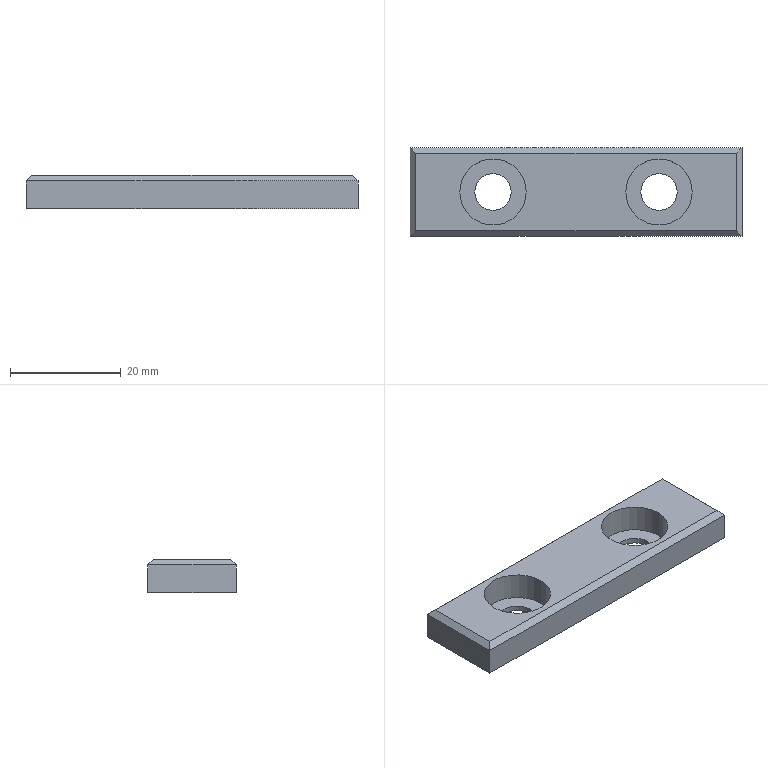Part | SolidWorks | features Cut 2, Chamfer 1, Extrusion 1, LPattern 1 | 1 solid | 20 faces | box 60 x 16 x 6 mm | volume 4486 mm3 | plane 12 | cylinder 8 | commonest cylinder face diameters 6.6 x4 12 x4
STEP:
#1=CARTESIAN_POINT('',(26.372,-2.26,1.));
#2=VERTEX_POINT('',#1);
#3=CARTESIAN_POINT('',(38.372,-2.26,1.));
#4=VERTEX_POINT('',#3);
#5=CARTESIAN_POINT('',(32.372,-2.26,1.));
#6=DIRECTION('',(0.,0.,1.));
#7=DIRECTION('',(1.,0.,0.));
#8=AXIS2_PLACEMENT_3D('',#5,#6,#7);
#9=CIRCLE('',#8,6.);
#10=EDGE_CURVE('',#2,#4,#9,.T.);
#11=ORIENTED_EDGE('',*,*,#10,.F.);
#12=CARTESIAN_POINT('',(26.372,-2.26,6.));
#13=VERTEX_POINT('',#12);
#14=CARTESIAN_POINT('',(26.372,-2.26,1.));
#15=DIRECTION('',(0.,0.,1.));
#16=VECTOR('',#15,1000.);
#17=LINE('',#14,#16);
#18=EDGE_CURVE('',#2,#13,#17,.T.);
#19=ORIENTED_EDGE('',*,*,#18,.T.);
#20=CARTESIAN_POINT('',(38.372,-2.26,6.));
#21=VERTEX_POINT('',#20);
#22=CARTESIAN_POINT('',(32.372,-2.26,6.));
#23=DIRECTION('',(0.,0.,1.));
#24=DIRECTION('',(1.,0.,0.));
#25=AXIS2_PLACEMENT_3D('',#22,#23,#24);
#26=CIRCLE('',#25,6.);
#27=EDGE_CURVE('',#13,#21,#26,.T.);
#28=ORIENTED_EDGE('',*,*,#27,.T.);
#29=CARTESIAN_POINT('',(38.372,-2.26,1.));
#30=DIRECTION('',(0.,0.,1.));
#31=VECTOR('',#30,1000.);
#32=LINE('',#29,#31);
#33=EDGE_CURVE('',#4,#21,#32,.T.);
#34=ORIENTED_EDGE('',*,*,#33,.F.);
#35=EDGE_LOOP('',(#11,#19,#28,#34));
#36=FACE_OUTER_BOUND('',#35,.T.);
#37=CARTESIAN_POINT('',(32.372,-2.26,1.));
#38=DIRECTION('',(0.,0.,1.));
#39=DIRECTION('',(1.,0.,0.));
#40=AXIS2_PLACEMENT_3D('',#37,#38,#39);
#41=CYLINDRICAL_SURFACE('',#40,6.);
#42=ADVANCED_FACE('',(#36),#41,.F.);
#43=CARTESIAN_POINT('',(-3.628,-2.26,1.));
#44=VERTEX_POINT('',#43);
#45=CARTESIAN_POINT('',(8.372,-2.26,1.));
#46=VERTEX_POINT('',#45);
#47=CARTESIAN_POINT('',(2.372,-2.26,1.));
#48=DIRECTION('',(0.,0.,1.));
#49=DIRECTION('',(1.,0.,0.));
#50=AXIS2_PLACEMENT_3D('',#47,#48,#49);
#51=CIRCLE('',#50,6.);
#52=EDGE_CURVE('',#44,#46,#51,.T.);
#53=ORIENTED_EDGE('',*,*,#52,.F.);
#54=CARTESIAN_POINT('',(-3.628,-2.26,6.));
#55=VERTEX_POINT('',#54);
#56=CARTESIAN_POINT('',(-3.628,-2.26,1.));
#57=DIRECTION('',(0.,0.,1.));
#58=VECTOR('',#57,1000.);
#59=LINE('',#56,#58);
#60=EDGE_CURVE('',#44,#55,#59,.T.);
#61=ORIENTED_EDGE('',*,*,#60,.T.);
#62=CARTESIAN_POINT('',(8.372,-2.26,6.));
#63=VERTEX_POINT('',#62);
#64=CARTESIAN_POINT('',(2.372,-2.26,6.));
#65=DIRECTION('',(0.,0.,1.));
#66=DIRECTION('',(1.,0.,0.));
#67=AXIS2_PLACEMENT_3D('',#64,#65,#66);
#68=CIRCLE('',#67,6.);
#69=EDGE_CURVE('',#55,#63,#68,.T.);
#70=ORIENTED_EDGE('',*,*,#69,.T.);
#71=CARTESIAN_POINT('',(8.372,-2.26,1.));
#72=DIRECTION('',(0.,0.,1.));
#73=VECTOR('',#72,1000.);
#74=LINE('',#71,#73);
#75=EDGE_CURVE('',#46,#63,#74,.T.);
#76=ORIENTED_EDGE('',*,*,#75,.F.);
#77=EDGE_LOOP('',(#53,#61,#70,#76));
#78=FACE_OUTER_BOUND('',#77,.T.);
#79=CARTESIAN_POINT('',(2.372,-2.26,1.));
#80=DIRECTION('',(0.,0.,1.));
#81=DIRECTION('',(1.,0.,0.));
#82=AXIS2_PLACEMENT_3D('',#79,#80,#81);
#83=CYLINDRICAL_SURFACE('',#82,6.);
#84=ADVANCED_FACE('',(#78),#83,.F.);
#85=CARTESIAN_POINT('',(-0.9282,-2.26,0.));
#86=VERTEX_POINT('',#85);
#87=CARTESIAN_POINT('',(5.672,-2.26,0.));
#88=VERTEX_POINT('',#87);
#89=CARTESIAN_POINT('',(2.372,-2.26,0.));
#90=DIRECTION('',(0.,0.,1.));
#91=DIRECTION('',(1.,0.,0.));
#92=AXIS2_PLACEMENT_3D('',#89,#90,#91);
#93=CIRCLE('',#92,3.3);
#94=EDGE_CURVE('',#86,#88,#93,.T.);
#95=ORIENTED_EDGE('',*,*,#94,.F.);
#96=CARTESIAN_POINT('',(-0.9282,-2.26,1.));
#97=VERTEX_POINT('',#96);
#98=CARTESIAN_POINT('',(-0.9282,-2.26,0.));
#99=DIRECTION('',(0.,0.,1.));
#100=VECTOR('',#99,1000.);
#101=LINE('',#98,#100);
#102=EDGE_CURVE('',#86,#97,#101,.T.);
#103=ORIENTED_EDGE('',*,*,#102,.T.);
#104=CARTESIAN_POINT('',(5.672,-2.26,1.));
#105=VERTEX_POINT('',#104);
#106=CARTESIAN_POINT('',(2.372,-2.26,1.));
#107=DIRECTION('',(0.,0.,-1.));
#108=DIRECTION('',(1.,0.,0.));
#109=AXIS2_PLACEMENT_3D('',#106,#107,#108);
#110=CIRCLE('',#109,3.3);
#111=EDGE_CURVE('',#105,#97,#110,.T.);
#112=ORIENTED_EDGE('',*,*,#111,.F.);
#113=CARTESIAN_POINT('',(5.672,-2.26,0.));
#114=DIRECTION('',(0.,0.,1.));
#115=VECTOR('',#114,1000.);
#116=LINE('',#113,#115);
#117=EDGE_CURVE('',#88,#105,#116,.T.);
#118=ORIENTED_EDGE('',*,*,#117,.F.);
#119=EDGE_LOOP('',(#95,#103,#112,#118));
#120=FACE_OUTER_BOUND('',#119,.T.);
#121=CARTESIAN_POINT('',(2.372,-2.26,0.));
#122=DIRECTION('',(0.,0.,1.));
#123=DIRECTION('',(1.,0.,0.));
#124=AXIS2_PLACEMENT_3D('',#121,#122,#123);
#125=CYLINDRICAL_SURFACE('',#124,3.3);
#126=ADVANCED_FACE('',(#120),#125,.F.);
#127=CARTESIAN_POINT('',(29.072,-2.26,0.));
#128=VERTEX_POINT('',#127);
#129=CARTESIAN_POINT('',(35.672,-2.26,0.));
#130=VERTEX_POINT('',#129);
#131=CARTESIAN_POINT('',(32.372,-2.26,0.));
#132=DIRECTION('',(0.,0.,1.));
#133=DIRECTION('',(1.,0.,0.));
#134=AXIS2_PLACEMENT_3D('',#131,#132,#133);
#135=CIRCLE('',#134,3.3);
#136=EDGE_CURVE('',#128,#130,#135,.T.);
#137=ORIENTED_EDGE('',*,*,#136,.F.);
#138=CARTESIAN_POINT('',(29.072,-2.26,1.));
#139=VERTEX_POINT('',#138);
#140=CARTESIAN_POINT('',(29.072,-2.26,0.));
#141=DIRECTION('',(0.,0.,1.));
#142=VECTOR('',#141,1000.);
#143=LINE('',#140,#142);
#144=EDGE_CURVE('',#128,#139,#143,.T.);
#145=ORIENTED_EDGE('',*,*,#144,.T.);
#146=CARTESIAN_POINT('',(35.672,-2.26,1.));
#147=VERTEX_POINT('',#146);
#148=CARTESIAN_POINT('',(32.372,-2.26,1.));
#149=DIRECTION('',(0.,0.,-1.));
#150=DIRECTION('',(1.,0.,0.));
#151=AXIS2_PLACEMENT_3D('',#148,#149,#150);
#152=CIRCLE('',#151,3.3);
#153=EDGE_CURVE('',#147,#139,#152,.T.);
#154=ORIENTED_EDGE('',*,*,#153,.F.);
#155=CARTESIAN_POINT('',(35.672,-2.26,0.));
#156=DIRECTION('',(0.,0.,1.));
#157=VECTOR('',#156,1000.);
#158=LINE('',#155,#157);
#159=EDGE_CURVE('',#130,#147,#158,.T.);
#160=ORIENTED_EDGE('',*,*,#159,.F.);
#161=EDGE_LOOP('',(#137,#145,#154,#160));
#162=FACE_OUTER_BOUND('',#161,.T.);
#163=CARTESIAN_POINT('',(32.372,-2.26,0.));
#164=DIRECTION('',(0.,0.,1.));
#165=DIRECTION('',(1.,0.,0.));
#166=AXIS2_PLACEMENT_3D('',#163,#164,#165);
#167=CYLINDRICAL_SURFACE('',#166,3.3);
#168=ADVANCED_FACE('',(#162),#167,.F.);
#169=ORIENTED_EDGE('',*,*,#144,.F.);
#170=CARTESIAN_POINT('',(32.372,-2.26,0.));
#171=DIRECTION('',(0.,0.,1.));
#172=DIRECTION('',(1.,0.,0.));
#173=AXIS2_PLACEMENT_3D('',#170,#171,#172);
#174=CIRCLE('',#173,3.3);
#175=EDGE_CURVE('',#130,#128,#174,.T.);
#176=ORIENTED_EDGE('',*,*,#175,.F.);
#177=ORIENTED_EDGE('',*,*,#159,.T.);
#178=CARTESIAN_POINT('',(32.372,-2.26,1.));
#179=DIRECTION('',(0.,0.,-1.));
#180=DIRECTION('',(1.,0.,0.));
#181=AXIS2_PLACEMENT_3D('',#178,#179,#180);
#182=CIRCLE('',#181,3.3);
#183=EDGE_CURVE('',#139,#147,#182,.T.);
#184=ORIENTED_EDGE('',*,*,#183,.F.);
#185=EDGE_LOOP('',(#169,#176,#177,#184));
#186=FACE_OUTER_BOUND('',#185,.T.);
#187=CARTESIAN_POINT('',(32.372,-2.26,0.));
#188=DIRECTION('',(0.,0.,1.));
#189=DIRECTION('',(1.,0.,0.));
#190=AXIS2_PLACEMENT_3D('',#187,#188,#189);
#191=CYLINDRICAL_SURFACE('',#190,3.3);
#192=ADVANCED_FACE('',(#186),#191,.F.);
#193=ORIENTED_EDGE('',*,*,#102,.F.);
#194=CARTESIAN_POINT('',(2.372,-2.26,0.));
#195=DIRECTION('',(0.,0.,1.));
#196=DIRECTION('',(1.,0.,0.));
#197=AXIS2_PLACEMENT_3D('',#194,#195,#196);
#198=CIRCLE('',#197,3.3);
#199=EDGE_CURVE('',#88,#86,#198,.T.);
#200=ORIENTED_EDGE('',*,*,#199,.F.);
#201=ORIENTED_EDGE('',*,*,#117,.T.);
#202=CARTESIAN_POINT('',(2.372,-2.26,1.));
#203=DIRECTION('',(0.,0.,-1.));
#204=DIRECTION('',(1.,0.,0.));
#205=AXIS2_PLACEMENT_3D('',#202,#203,#204);
#206=CIRCLE('',#205,3.3);
#207=EDGE_CURVE('',#97,#105,#206,.T.);
#208=ORIENTED_EDGE('',*,*,#207,.F.);
#209=EDGE_LOOP('',(#193,#200,#201,#208));
#210=FACE_OUTER_BOUND('',#209,.T.);
#211=CARTESIAN_POINT('',(2.372,-2.26,0.));
#212=DIRECTION('',(0.,0.,1.));
#213=DIRECTION('',(1.,0.,0.));
#214=AXIS2_PLACEMENT_3D('',#211,#212,#213);
#215=CYLINDRICAL_SURFACE('',#214,3.3);
#216=ADVANCED_FACE('',(#210),#215,.F.);
#217=CARTESIAN_POINT('',(-12.628,-10.26,5.));
#218=VERTEX_POINT('',#217);
#219=CARTESIAN_POINT('',(-12.628,-10.26,0.));
#220=VERTEX_POINT('',#219);
#221=CARTESIAN_POINT('',(-12.628,-10.26,6.));
#222=DIRECTION('',(0.,0.,-1.));
#223=VECTOR('',#222,1000.);
#224=LINE('',#221,#223);
#225=EDGE_CURVE('',#218,#220,#224,.T.);
#226=ORIENTED_EDGE('',*,*,#225,.F.);
#227=CARTESIAN_POINT('',(-12.628,5.74,5.));
#228=VERTEX_POINT('',#227);
#229=CARTESIAN_POINT('',(-12.628,5.74,5.));
#230=DIRECTION('',(0.,1.,0.));
#231=VECTOR('',#230,1000.);
#232=LINE('',#229,#231);
#233=EDGE_CURVE('',#218,#228,#232,.T.);
#234=ORIENTED_EDGE('',*,*,#233,.T.);
#235=CARTESIAN_POINT('',(-12.628,5.74,0.));
#236=VERTEX_POINT('',#235);
#237=CARTESIAN_POINT('',(-12.628,5.74,6.));
#238=DIRECTION('',(0.,0.,-1.));
#239=VECTOR('',#238,1000.);
#240=LINE('',#237,#239);
#241=EDGE_CURVE('',#228,#236,#240,.T.);
#242=ORIENTED_EDGE('',*,*,#241,.T.);
#243=CARTESIAN_POINT('',(-12.628,5.74,0.));
#244=DIRECTION('',(0.,-1.,0.));
#245=VECTOR('',#244,1000.);
#246=LINE('',#243,#245);
#247=EDGE_CURVE('',#236,#220,#246,.T.);
#248=ORIENTED_EDGE('',*,*,#247,.T.);
#249=EDGE_LOOP('',(#226,#234,#242,#248));
#250=FACE_OUTER_BOUND('',#249,.T.);
#251=CARTESIAN_POINT('',(-12.628,5.74,6.));
#252=DIRECTION('',(1.,0.,0.));
#253=DIRECTION('',(0.,1.,0.));
#254=AXIS2_PLACEMENT_3D('',#251,#252,#253);
#255=PLANE('',#254);
#256=ADVANCED_FACE('',(#250),#255,.F.);
#257=CARTESIAN_POINT('',(47.372,-10.26,5.));
#258=VERTEX_POINT('',#257);
#259=CARTESIAN_POINT('',(47.372,-10.26,0.));
#260=VERTEX_POINT('',#259);
#261=CARTESIAN_POINT('',(47.372,-10.26,6.));
#262=DIRECTION('',(0.,0.,-1.));
#263=VECTOR('',#262,1000.);
#264=LINE('',#261,#263);
#265=EDGE_CURVE('',#258,#260,#264,.T.);
#266=ORIENTED_EDGE('',*,*,#265,.F.);
#267=CARTESIAN_POINT('',(-12.628,-10.26,5.));
#268=DIRECTION('',(-1.,0.,0.));
#269=VECTOR('',#268,1000.);
#270=LINE('',#267,#269);
#271=EDGE_CURVE('',#258,#218,#270,.T.);
#272=ORIENTED_EDGE('',*,*,#271,.T.);
#273=ORIENTED_EDGE('',*,*,#225,.T.);
#274=CARTESIAN_POINT('',(-12.628,-10.26,0.));
#275=DIRECTION('',(1.,0.,0.));
#276=VECTOR('',#275,1000.);
#277=LINE('',#274,#276);
#278=EDGE_CURVE('',#220,#260,#277,.T.);
#279=ORIENTED_EDGE('',*,*,#278,.T.);
#280=EDGE_LOOP('',(#266,#272,#273,#279));
#281=FACE_OUTER_BOUND('',#280,.T.);
#282=CARTESIAN_POINT('',(-12.628,-10.26,6.));
#283=DIRECTION('',(0.,1.,0.));
#284=DIRECTION('',(0.,0.,1.));
#285=AXIS2_PLACEMENT_3D('',#282,#283,#284);
#286=PLANE('',#285);
#287=ADVANCED_FACE('',(#281),#286,.F.);
#288=CARTESIAN_POINT('',(47.372,5.74,5.));
#289=VERTEX_POINT('',#288);
#290=CARTESIAN_POINT('',(47.372,5.74,0.));
#291=VERTEX_POINT('',#290);
#292=CARTESIAN_POINT('',(47.372,5.74,6.));
#293=DIRECTION('',(0.,0.,-1.));
#294=VECTOR('',#293,1000.);
#295=LINE('',#292,#294);
#296=EDGE_CURVE('',#289,#291,#295,.T.);
#297=ORIENTED_EDGE('',*,*,#296,.F.);
#298=CARTESIAN_POINT('',(47.372,-10.26,5.));
#299=DIRECTION('',(0.,-1.,0.));
#300=VECTOR('',#299,1000.);
#301=LINE('',#298,#300);
#302=EDGE_CURVE('',#289,#258,#301,.T.);
#303=ORIENTED_EDGE('',*,*,#302,.T.);
#304=ORIENTED_EDGE('',*,*,#265,.T.);
#305=CARTESIAN_POINT('',(47.372,5.74,0.));
#306=DIRECTION('',(0.,1.,0.));
#307=VECTOR('',#306,1000.);
#308=LINE('',#305,#307);
#309=EDGE_CURVE('',#260,#291,#308,.T.);
#310=ORIENTED_EDGE('',*,*,#309,.T.);
#311=EDGE_LOOP('',(#297,#303,#304,#310));
#312=FACE_OUTER_BOUND('',#311,.T.);
#313=CARTESIAN_POINT('',(47.372,5.74,6.));
#314=DIRECTION('',(-1.,0.,0.));
#315=DIRECTION('',(0.,0.,1.));
#316=AXIS2_PLACEMENT_3D('',#313,#314,#315);
#317=PLANE('',#316);
#318=ADVANCED_FACE('',(#312),#317,.F.);
#319=ORIENTED_EDGE('',*,*,#241,.F.);
#320=CARTESIAN_POINT('',(47.372,5.74,5.));
#321=DIRECTION('',(1.,0.,0.));
#322=VECTOR('',#321,1000.);
#323=LINE('',#320,#322);
#324=EDGE_CURVE('',#228,#289,#323,.T.);
#325=ORIENTED_EDGE('',*,*,#324,.T.);
#326=ORIENTED_EDGE('',*,*,#296,.T.);
#327=CARTESIAN_POINT('',(-12.628,5.74,0.));
#328=DIRECTION('',(-1.,0.,0.));
#329=VECTOR('',#328,1000.);
#330=LINE('',#327,#329);
#331=EDGE_CURVE('',#291,#236,#330,.T.);
#332=ORIENTED_EDGE('',*,*,#331,.T.);
#333=EDGE_LOOP('',(#319,#325,#326,#332));
#334=FACE_OUTER_BOUND('',#333,.T.);
#335=CARTESIAN_POINT('',(-12.628,5.74,6.));
#336=DIRECTION('',(0.,-1.,0.));
#337=DIRECTION('',(0.,0.,-1.));
#338=AXIS2_PLACEMENT_3D('',#335,#336,#337);
#339=PLANE('',#338);
#340=ADVANCED_FACE('',(#334),#339,.F.);
#341=CARTESIAN_POINT('',(46.372,-9.26,6.));
#342=VERTEX_POINT('',#341);
#343=CARTESIAN_POINT('',(46.372,4.74,6.));
#344=VERTEX_POINT('',#343);
#345=CARTESIAN_POINT('',(46.372,5.74,6.));
#346=DIRECTION('',(0.,1.,0.));
#347=VECTOR('',#346,1000.);
#348=LINE('',#345,#347);
#349=EDGE_CURVE('',#342,#344,#348,.T.);
#350=ORIENTED_EDGE('',*,*,#349,.T.);
#351=CARTESIAN_POINT('',(-11.628,4.74,6.));
#352=VERTEX_POINT('',#351);
#353=CARTESIAN_POINT('',(-12.628,4.74,6.));
#354=DIRECTION('',(-1.,0.,0.));
#355=VECTOR('',#354,1000.);
#356=LINE('',#353,#355);
#357=EDGE_CURVE('',#344,#352,#356,.T.);
#358=ORIENTED_EDGE('',*,*,#357,.T.);
#359=CARTESIAN_POINT('',(-11.628,-9.26,6.));
#360=VERTEX_POINT('',#359);
#361=CARTESIAN_POINT('',(-11.628,-10.26,6.));
#362=DIRECTION('',(0.,-1.,0.));
#363=VECTOR('',#362,1000.);
#364=LINE('',#361,#363);
#365=EDGE_CURVE('',#352,#360,#364,.T.);
#366=ORIENTED_EDGE('',*,*,#365,.T.);
#367=CARTESIAN_POINT('',(47.372,-9.26,6.));
#368=DIRECTION('',(1.,0.,0.));
#369=VECTOR('',#368,1000.);
#370=LINE('',#367,#369);
#371=EDGE_CURVE('',#360,#342,#370,.T.);
#372=ORIENTED_EDGE('',*,*,#371,.T.);
#373=EDGE_LOOP('',(#350,#358,#366,#372));
#374=FACE_OUTER_BOUND('',#373,.T.);
#375=CARTESIAN_POINT('',(32.372,-2.26,6.));
#376=DIRECTION('',(0.,0.,1.));
#377=DIRECTION('',(1.,0.,0.));
#378=AXIS2_PLACEMENT_3D('',#375,#376,#377);
#379=CIRCLE('',#378,6.);
#380=EDGE_CURVE('',#21,#13,#379,.T.);
#381=ORIENTED_EDGE('',*,*,#380,.F.);
#382=ORIENTED_EDGE('',*,*,#27,.F.);
#383=EDGE_LOOP('',(#381,#382));
#384=FACE_BOUND('',#383,.T.);
#385=CARTESIAN_POINT('',(2.372,-2.26,6.));
#386=DIRECTION('',(0.,0.,1.));
#387=DIRECTION('',(1.,0.,0.));
#388=AXIS2_PLACEMENT_3D('',#385,#386,#387);
#389=CIRCLE('',#388,6.);
#390=EDGE_CURVE('',#63,#55,#389,.T.);
#391=ORIENTED_EDGE('',*,*,#390,.F.);
#392=ORIENTED_EDGE('',*,*,#69,.F.);
#393=EDGE_LOOP('',(#391,#392));
#394=FACE_BOUND('',#393,.T.);
#395=CARTESIAN_POINT('',(-12.628,-10.26,6.));
#396=DIRECTION('',(0.,0.,1.));
#397=DIRECTION('',(1.,0.,0.));
#398=AXIS2_PLACEMENT_3D('',#395,#396,#397);
#399=PLANE('',#398);
#400=ADVANCED_FACE('',(#374,#384,#394),#399,.T.);
#401=ORIENTED_EDGE('',*,*,#175,.T.);
#402=ORIENTED_EDGE('',*,*,#136,.T.);
#403=EDGE_LOOP('',(#401,#402));
#404=FACE_BOUND('',#403,.T.);
#405=ORIENTED_EDGE('',*,*,#199,.T.);
#406=ORIENTED_EDGE('',*,*,#94,.T.);
#407=EDGE_LOOP('',(#405,#406));
#408=FACE_BOUND('',#407,.T.);
#409=ORIENTED_EDGE('',*,*,#247,.F.);
#410=ORIENTED_EDGE('',*,*,#331,.F.);
#411=ORIENTED_EDGE('',*,*,#309,.F.);
#412=ORIENTED_EDGE('',*,*,#278,.F.);
#413=EDGE_LOOP('',(#409,#410,#411,#412));
#414=FACE_OUTER_BOUND('',#413,.T.);
#415=CARTESIAN_POINT('',(-12.628,-10.26,0.));
#416=DIRECTION('',(0.,0.,1.));
#417=DIRECTION('',(1.,0.,0.));
#418=AXIS2_PLACEMENT_3D('',#415,#416,#417);
#419=PLANE('',#418);
#420=ADVANCED_FACE('',(#404,#408,#414),#419,.F.);
#421=CARTESIAN_POINT('',(2.372,-2.26,1.));
#422=DIRECTION('',(0.,0.,1.));
#423=DIRECTION('',(1.,0.,0.));
#424=AXIS2_PLACEMENT_3D('',#421,#422,#423);
#425=CIRCLE('',#424,6.);
#426=EDGE_CURVE('',#46,#44,#425,.T.);
#427=ORIENTED_EDGE('',*,*,#426,.T.);
#428=ORIENTED_EDGE('',*,*,#52,.T.);
#429=EDGE_LOOP('',(#427,#428));
#430=FACE_OUTER_BOUND('',#429,.T.);
#431=ORIENTED_EDGE('',*,*,#111,.T.);
#432=ORIENTED_EDGE('',*,*,#207,.T.);
#433=EDGE_LOOP('',(#431,#432));
#434=FACE_BOUND('',#433,.T.);
#435=CARTESIAN_POINT('',(2.372,-2.26,1.));
#436=DIRECTION('',(0.,0.,1.));
#437=DIRECTION('',(1.,0.,0.));
#438=AXIS2_PLACEMENT_3D('',#435,#436,#437);
#439=PLANE('',#438);
#440=ADVANCED_FACE('',(#430,#434),#439,.T.);
#441=ORIENTED_EDGE('',*,*,#60,.F.);
#442=ORIENTED_EDGE('',*,*,#426,.F.);
#443=ORIENTED_EDGE('',*,*,#75,.T.);
#444=ORIENTED_EDGE('',*,*,#390,.T.);
#445=EDGE_LOOP('',(#441,#442,#443,#444));
#446=FACE_OUTER_BOUND('',#445,.T.);
#447=CARTESIAN_POINT('',(2.372,-2.26,1.));
#448=DIRECTION('',(0.,0.,1.));
#449=DIRECTION('',(1.,0.,0.));
#450=AXIS2_PLACEMENT_3D('',#447,#448,#449);
#451=CYLINDRICAL_SURFACE('',#450,6.);
#452=ADVANCED_FACE('',(#446),#451,.F.);
#453=CARTESIAN_POINT('',(32.372,-2.26,1.));
#454=DIRECTION('',(0.,0.,1.));
#455=DIRECTION('',(1.,0.,0.));
#456=AXIS2_PLACEMENT_3D('',#453,#454,#455);
#457=CIRCLE('',#456,6.);
#458=EDGE_CURVE('',#4,#2,#457,.T.);
#459=ORIENTED_EDGE('',*,*,#458,.T.);
#460=ORIENTED_EDGE('',*,*,#10,.T.);
#461=EDGE_LOOP('',(#459,#460));
#462=FACE_OUTER_BOUND('',#461,.T.);
#463=ORIENTED_EDGE('',*,*,#153,.T.);
#464=ORIENTED_EDGE('',*,*,#183,.T.);
#465=EDGE_LOOP('',(#463,#464));
#466=FACE_BOUND('',#465,.T.);
#467=CARTESIAN_POINT('',(32.372,-2.26,1.));
#468=DIRECTION('',(0.,0.,1.));
#469=DIRECTION('',(1.,0.,0.));
#470=AXIS2_PLACEMENT_3D('',#467,#468,#469);
#471=PLANE('',#470);
#472=ADVANCED_FACE('',(#462,#466),#471,.T.);
#473=ORIENTED_EDGE('',*,*,#18,.F.);
#474=ORIENTED_EDGE('',*,*,#458,.F.);
#475=ORIENTED_EDGE('',*,*,#33,.T.);
#476=ORIENTED_EDGE('',*,*,#380,.T.);
#477=EDGE_LOOP('',(#473,#474,#475,#476));
#478=FACE_OUTER_BOUND('',#477,.T.);
#479=CARTESIAN_POINT('',(32.372,-2.26,1.));
#480=DIRECTION('',(0.,0.,1.));
#481=DIRECTION('',(1.,0.,0.));
#482=AXIS2_PLACEMENT_3D('',#479,#480,#481);
#483=CYLINDRICAL_SURFACE('',#482,6.);
#484=ADVANCED_FACE('',(#478),#483,.F.);
#485=CARTESIAN_POINT('',(-11.962,-9.594,5.667));
#486=DIRECTION('',(0.5774,0.5774,0.5774));
#487=VECTOR('',#486,1000.);
#488=LINE('',#485,#487);
#489=EDGE_CURVE('',#218,#360,#488,.T.);
#490=ORIENTED_EDGE('',*,*,#489,.F.);
#491=ORIENTED_EDGE('',*,*,#271,.F.);
#492=CARTESIAN_POINT('',(46.705,-9.594,5.667));
#493=DIRECTION('',(0.5774,-0.5774,-0.5774));
#494=VECTOR('',#493,1000.);
#495=LINE('',#492,#494);
#496=EDGE_CURVE('',#342,#258,#495,.T.);
#497=ORIENTED_EDGE('',*,*,#496,.F.);
#498=ORIENTED_EDGE('',*,*,#371,.F.);
#499=EDGE_LOOP('',(#490,#491,#497,#498));
#500=FACE_OUTER_BOUND('',#499,.T.);
#501=CARTESIAN_POINT('',(-12.628,-9.26,6.));
#502=DIRECTION('',(0.,-0.7071,0.7071));
#503=DIRECTION('',(0.,-0.7071,-0.7071));
#504=AXIS2_PLACEMENT_3D('',#501,#502,#503);
#505=PLANE('',#504);
#506=ADVANCED_FACE('',(#500),#505,.T.);
#507=ORIENTED_EDGE('',*,*,#496,.T.);
#508=ORIENTED_EDGE('',*,*,#302,.F.);
#509=CARTESIAN_POINT('',(41.372,-0.2605,11.));
#510=DIRECTION('',(0.5774,0.5774,-0.5774));
#511=VECTOR('',#510,1000.);
#512=LINE('',#509,#511);
#513=EDGE_CURVE('',#344,#289,#512,.T.);
#514=ORIENTED_EDGE('',*,*,#513,.F.);
#515=ORIENTED_EDGE('',*,*,#349,.F.);
#516=EDGE_LOOP('',(#507,#508,#514,#515));
#517=FACE_OUTER_BOUND('',#516,.T.);
#518=CARTESIAN_POINT('',(46.372,-10.26,6.));
#519=DIRECTION('',(0.7071,0.,0.7071));
#520=DIRECTION('',(0.7071,0.,-0.7071));
#521=AXIS2_PLACEMENT_3D('',#518,#519,#520);
#522=PLANE('',#521);
#523=ADVANCED_FACE('',(#517),#522,.T.);
#524=ORIENTED_EDGE('',*,*,#489,.T.);
#525=ORIENTED_EDGE('',*,*,#365,.F.);
#526=CARTESIAN_POINT('',(-6.628,-0.2605,11.));
#527=DIRECTION('',(0.5774,-0.5774,0.5774));
#528=VECTOR('',#527,1000.);
#529=LINE('',#526,#528);
#530=EDGE_CURVE('',#228,#352,#529,.T.);
#531=ORIENTED_EDGE('',*,*,#530,.F.);
#532=ORIENTED_EDGE('',*,*,#233,.F.);
#533=EDGE_LOOP('',(#524,#525,#531,#532));
#534=FACE_OUTER_BOUND('',#533,.T.);
#535=CARTESIAN_POINT('',(-11.628,-10.26,6.));
#536=DIRECTION('',(-0.7071,0.,0.7071));
#537=DIRECTION('',(0.7071,0.,0.7071));
#538=AXIS2_PLACEMENT_3D('',#535,#536,#537);
#539=PLANE('',#538);
#540=ADVANCED_FACE('',(#534),#539,.T.);
#541=ORIENTED_EDGE('',*,*,#513,.T.);
#542=ORIENTED_EDGE('',*,*,#324,.F.);
#543=ORIENTED_EDGE('',*,*,#530,.T.);
#544=ORIENTED_EDGE('',*,*,#357,.F.);
#545=EDGE_LOOP('',(#541,#542,#543,#544));
#546=FACE_OUTER_BOUND('',#545,.T.);
#547=CARTESIAN_POINT('',(-12.628,4.74,6.));
#548=DIRECTION('',(0.,0.7071,0.7071));
#549=DIRECTION('',(0.,-0.7071,0.7071));
#550=AXIS2_PLACEMENT_3D('',#547,#548,#549);
#551=PLANE('',#550);
#552=ADVANCED_FACE('',(#546),#551,.T.);
#553=CLOSED_SHELL('',(#42,#84,#126,#168,#192,#216,#256,#287,#318,#340,#400,#420,#440,#452,#472,#484,#506,#523,#540,#552));
#554=MANIFOLD_SOLID_BREP('',#553);
#555=CARTESIAN_POINT('',(0.,0.,0.));
#556=DIRECTION('',(0.,0.,1.));
#557=DIRECTION('',(1.,0.,0.));
#558=AXIS2_PLACEMENT_3D('',#555,#556,#557);
#559=(LENGTH_UNIT()NAMED_UNIT(*)SI_UNIT(.MILLI.,.METRE.));
#560=UNCERTAINTY_MEASURE_WITH_UNIT(LENGTH_MEASURE(0.00001),#559,'','');
#561=(NAMED_UNIT(*)PLANE_ANGLE_UNIT()SI_UNIT($,.RADIAN.));
#562=(NAMED_UNIT(*)SI_UNIT($,.STERADIAN.)SOLID_ANGLE_UNIT());
#563=(GEOMETRIC_REPRESENTATION_CONTEXT(3)GLOBAL_UNCERTAINTY_ASSIGNED_CONTEXT((#560))GLOBAL_UNIT_ASSIGNED_CONTEXT((#559,#561,#562))REPRESENTATION_CONTEXT('',''));
#564=ADVANCED_BREP_SHAPE_REPRESENTATION('',(#554,#558),#563);